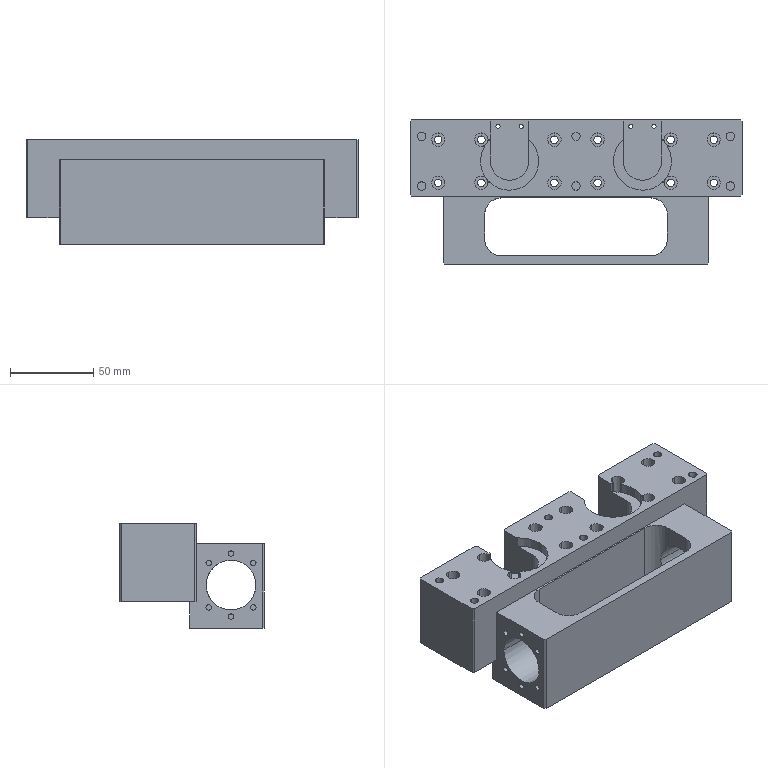Part | 1 solid | 219 faces | box 200 x 87 x 63 mm | volume 462867 mm3 | cylinder 144 | plane 75 | commonest cylinder face diameters 3.3 x42 4.5 x24 8 x24 1 x12 5.1 x12 2.5 x8